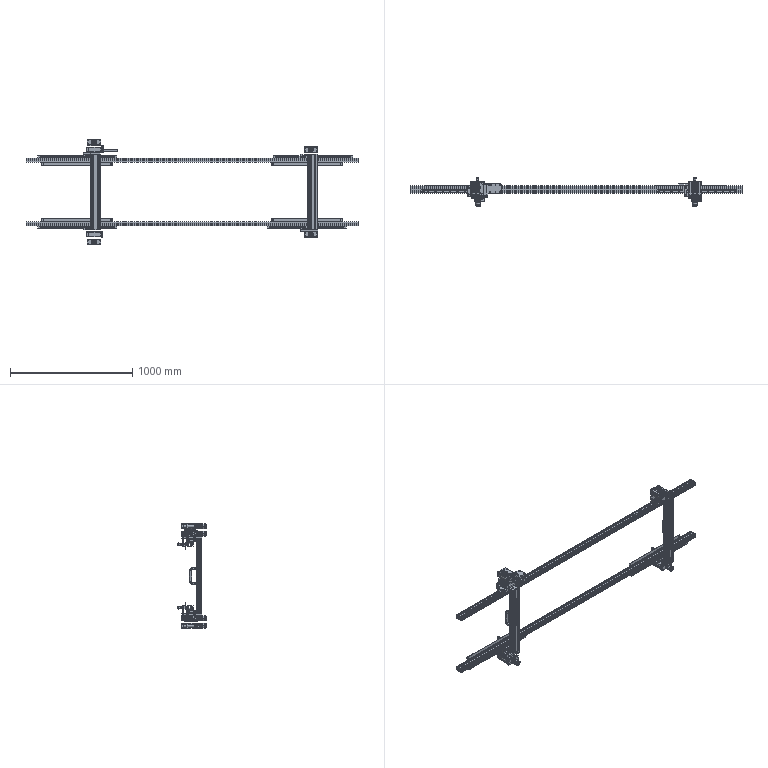Part | SolidWorks | features ReferencePattern 36, MirrorCompFeat 3, CompositeCurve 2, LocalLPattern 2 | 119 solids | 8109 faces | volume 11952575 mm3 | plane 2975 | cylinder 2694 | torus 896 | cone 864 | sphere 512 | spline 168 | commonest cylinder face diameters 0.4 x204 2 x176 0.8 x168 11 x146 5 x142 4 x109